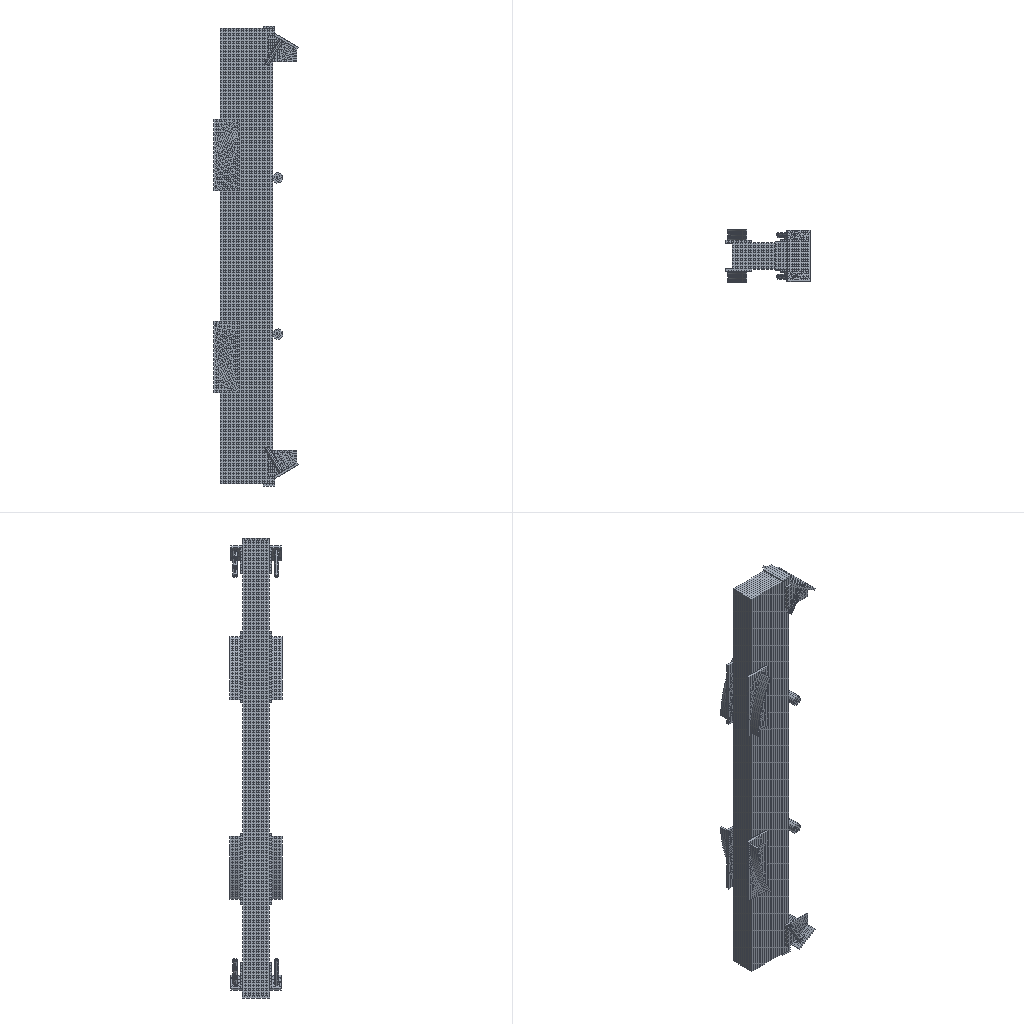Simulation study | abaqus
Set-up summary:
category,name,step,type,value,unit,region
solver,abaqus
solver,version,,,Abaqus/Explicit 2020
units,not stated in the deck,,not stated
analysis,deck,,transient,transient
load_step,Step-1,Step-1,transient
load_step,requested,,,1
mesh,nodes,,,51207
mesh,elements,,,41180
element_type,T3D2,,truss,1847
element_type,C3D8R,,solid,39333
load,load commands in deck,,count,1
bc,support commands in deck,,count,11
material,C40,,in results
material,CFRP,,in results
material,GANGBAN,,in results
material,GANGJIN,,in results
material,GUJIN,,in results
check,setup vs results,,match,"per instance, exact: element labels, types and connectivity; labels of the nodes the elements use; coordinates of those nodes at SINGLE_PRECISION in 10 of 15 instance(s)"
Abaqus input file, long lists of numbers shortened:
*Heading
** Job name: Job-2 Model name: Model-1
** Generated by: Abaqus/CAE 2020
*Preprint, echo=NO, model=NO, history=NO, contact=NO
**
** PARTS
**
*Part, name=ban
*Node
      1,   526.642,  -13.109,         -80.
      2,   526.642,  -23.112,         -80.
** (970 more lines like these left out)
*Element, type=C3D8R
  1, 118, 122, 341, 269,   1,   2,  17,  64
  2, 269, 341, 342, 270,  64,  17,  18,  63
** (441 more lines like these left out)
*Nset, nset=Set-1, generate
   1,  972,    1
*Elset, elset=Set-1, generate
   1,  443,    1
** Section: gangban
*Solid Section, elset=Set-1, material=gangban
,
*End Part
**
*Part, name=ban-Copy
*Node
      1,   507.77,  -151.344,         -80.
      2,   502.692,  -159.959,         -80.
** (960 more lines like these left out)
*Element, type=C3D8R
  1, 118, 122, 341, 269,   1,   2,  17,  64
  2, 269, 341, 342, 270,  64,  17,  18,  63
** (436 more lines like these left out)
*Nset, nset=Set-1, generate
   1,  962,    1
*Elset, elset=Set-1, generate
   1,  438,    1
** Section: gangban
*Solid Section, elset=Set-1, material=gangban
,
*End Part
**
*Part, name=con
*Node
      1,           0.,           0.,           0.
      2,          20.,           0.,           0.
** (40654 more lines like these left out)
*Element, type=C3D8R
    1,   232,   233,   254,   253,     1,     2,    23,    22
    2,   233,   234,   255,   254,     2,     3,    24,    23
** (34998 more lines like these left out)
*Nset, nset=Set-1, generate
     1,  40656,      1
*Elset, elset=Set-1, generate
     1,  35000,      1
** Section: con
*Solid Section, elset=Set-1, material=c40
,
*End Part
**
*Part, name=jin-final
*Node
      1,         365.,        -180.,        3250.
      2,          35.,        -180.,        3250.
** (1401 more lines like these left out)
*Element, type=T3D2
 1,  2, 73
 2, 73, 74
** (1461 more lines like these left out)
*Nset, nset=Set-1
    1,    2,    3,    4,    5,    6,    7,    8,    9,   10,   11,   12,   13,   14,   15,   16
   17,   18,   19,   20,   21,   22,   23,   24,   25,   26,   27,   28,   29,   30,   31,   32
** (54 more lines like these left out)
*Elset, elset=Set-1
   18,   19,   20,   21,   22,   23,   24,   25,   26,   27,   28,   29,   30,   31,   32,   33
   34,   35,   36,   37,   38,   39,   40,   41,   59,   60,   61,   62,   63,   64,   65,   66
** (56 more lines like these left out)
*Nset, nset=Set-2
    1,    2,    3,    5,    7,   10,   11,   12,   13,   14,   15,   16,   17,   18,   19,   20
   21,   22,   23,   24,   25,   26,   27,   28,   29,   30,   31,   32,   33,   34,   35,   36
** (34 more lines like these left out)
*Elset, elset=Set-2
    1,    2,    3,    4,    5,    6,    7,    8,    9,   10,   11,   12,   13,   14,   15,   16
   17,   42,   43,   44,   45,   46,   47,   48,   49,   50,   51,   52,   53,   54,   55,   56
** (32 more lines like these left out)
** Section: gujin
*Solid Section, elset=Set-2, material=gujin
50.5,
** Section: gangjin
*Solid Section, elset=Set-1, material=gangjin
201.,
*End Part
**
*Part, name=mao
*Node
      1,   5.039,   9.778,         220.
      2,   8.131,   15.496,         220.
** (238 more lines like these left out)
*Element, type=C3D8R
  1,  21,  22,  32,  33,   1,   2,  12,  13
  2,  33,  32,  23,  24,  13,  12,   3,   4
** (108 more lines like these left out)
*Nset, nset=Set-1, generate
   1,  240,    1
*Elset, elset=Set-1, generate
   1,  110,    1
** Section: gangban
*Solid Section, elset=Set-1, material=gangban
,
*End Part
**
*Part, name=rig
*Node
      1,   37.278,  -14.504,           0.
      2,   39.879,   3.106,           0.
** (606 more lines like these left out)
*Element, type=C3D8R
  1,  68,  50,  49,  54,  30,  12,  11,  16
  2,  54,  49,  48,  69,  16,  11,  10,  31
** (448 more lines like these left out)
*Nset, nset=Set-1, generate
   1,  608,    1
*Elset, elset=Set-1, generate
   1,  450,    1
** Section: gangban
*Solid Section, elset=Set-1, material=gangban
,
*End Part
**
*Part, name=xian
*Node
      1,  -1897.019,   560.759,           0.
      2,  -1121.676,    103.766,           0.
** (191 more lines like these left out)
*Element, type=T3D2
 1,  2,  7
 2,  7,  8
** (190 more lines like these left out)
*Nset, nset=Set-1, generate
   1,  193,    1
*Elset, elset=Set-1, generate
   1,  192,    1
*Nset, nset=Set-6, generate
   1,  193,    1
*Elset, elset=Set-6, generate
   1,  192,    1
*Orientation, name=Ori-6
          1.,           0.,           0.,           0.,           1.,           0.
1, 0.
** Section: cfrp
*Solid Section, elset=Set-1, material=cfrp
380.,
*End Part
**
*Part, name=zhifan-final
*Node
      1,         416.,           5.,          59.
      2,   424.112,           5.,    45.209
** (2716 more lines like these left out)
*Element, type=C3D8R
  1,  160,  170, 1003,  913,    1,    2,  105,  124
  2,  913, 1003, 1004,  914,  124,  105,  106,  123
** (1229 more lines like these left out)
*Nset, nset=Set-1, generate
    1,  2718,     1
*Elset, elset=Set-1, generate
    1,  1231,     1
** Section: gangban
*Solid Section, elset=Set-1, material=gangban
,
*End Part
**
**
** ASSEMBLY
**
*Assembly, name=Assembly
**
*Instance, name=ban-1, part=ban
        -50.,          20.,         700.
        -50.,          20.,         700., -49.423, 19.423, 700.577,         120.
*End Instance
**
*Instance, name=con-1, part=con
*End Instance
**
*Instance, name=ban-Copy-1, part=ban-Copy
        -50.,          20.,        2250.
        -50.,          20.,        2250., -49.423, 19.423, 2250.577,         120.
*End Instance
**
*Instance, name=ban-2, part=ban
        -50.,        -220.,        2800.
        -50.,        -220.,        2800., -50.577, -219.423, 2800.577,         120.
*End Instance
**
*Instance, name=ban-Copy-2, part=ban-Copy
        -50.,        -220.,        1250.
        -50.,        -220.,        1250., -50.577, -219.423, 1250.577,         120.
*End Instance
**
*Instance, name=rig-1, part=rig
        440.,          50.,        1150.
        440.,          50.,        1150., 441.,          50.,        1150., 90.
*End Instance
**
*Instance, name=rig-1-lin-2-1, part=rig
        440.,          50.,        2350.
        440.,          50.,        2350., 441.,          50.,        2350., 90.
*End Instance
**
*Instance, name=zhifan-final-1, part=zhifan-final
*End Instance
**
*Instance, name=xian-1, part=xian
  -23.419,          60.,  1636.086
  -23.419,          60.,  1636.086, -22.842, 60.577, 1635.508,         120.
*End Instance
**
*Instance, name=xian-1-lin-2-1, part=xian
  -23.419,        -260.,  1636.086
  -23.419,        -260.,  1636.086, -22.842, -259.423, 1635.508,         120.
*End Instance
**
*Instance, name=mao-1, part=mao
354.08, 60., 277.816
354.08, 60., 277.816, 354.08, 61., 277.816, 149.485
*End Instance
**
*Instance, name=mao-1-lin-2-1, part=mao
354.08,        -260., 277.816
354.08,        -260., 277.816, 354.08, -259., 277.816, 149.485
*End Instance
**
*Instance, name=mao-2, part=mao
465.79, 60., 3411.712
465.79, 60., 3411.712, 465.79, 61., 3411.712, 210.515
*End Instance
**
*Instance, name=mao-2-lin-2-1, part=mao
465.79,        -260., 3411.712
465.79,        -260., 3411.712, 465.79, -259., 3411.712, 210.515
*End Instance
**
*Instance, name=jin-final-1, part=jin-final
*End Instance
**
*Node
      1,         400.,        -100.,        1750.
*Nset, nset=Set-3, instance=con-1
     1,    22,    43,    64,    85,   106,   127,   148,   169,   190,   211,   232,   253,   274,   295,   316
   337,   358,   379,   400,   421,   442,   463,   484,   505,   526,   547,   568,   589,   610,   631,   652
** (14 more lines like these left out)
*Elset, elset=Set-3, instance=con-1
     1,    21,    41,    61,    81,   101,   121,   141,   161,   181,   201,   221,   241,   261,   281,   301
   321,   341,   361,   381,   401,   421,   441,   461,   481,   501,   521,   541,   561,   581,   601,   621
** (11 more lines like these left out)
*Nset, nset=Set-4
 1,
*Nset, nset=Set-5, instance=jin-final-1, generate
    1,  1403,     1
*Elset, elset=Set-5, instance=jin-final-1, generate
    1,  1463,     1
*Nset, nset=Set-8, instance=xian-1, generate
   1,  193,    1
*Nset, nset=Set-8, instance=xian-1-lin-2-1, generate
   1,  193,    1
*Elset, elset=Set-8, instance=xian-1, generate
   1,  192,    1
*Elset, elset=Set-8, instance=xian-1-lin-2-1, generate
   1,  192,    1
*Nset, nset=Set-9, instance=xian-1
 1, 6
*Nset, nset=Set-9, instance=xian-1-lin-2-1
 1, 6
*Nset, nset=b_Set-1, instance=rig-1, generate
   1,  608,    1
*Nset, nset=b_Set-1, instance=rig-1-lin-2-1, generate
   1,  608,    1
*Elset, elset=b_Set-1, instance=rig-1, generate
   1,  450,    1
*Elset, elset=b_Set-1, instance=rig-1-lin-2-1, generate
   1,  450,    1
*Nset, nset=m_Set-6, instance=jin-final-1, generate
    1,  1403,     1
*Elset, elset=m_Set-6, instance=jin-final-1, generate
    1,  1463,     1
*Nset, nset=s_Set-6, instance=con-1, generate
     1,  40656,      1
*Elset, elset=s_Set-6, instance=con-1, generate
     1,  35000,      1
*Nset, nset=_PickedSet87, internal
 1,
*Elset, elset=_m_Surf-1_S3, internal, instance=con-1
     1,     2,     3,     4,     5,     6,     7,     8,     9,    10,    11,    12,    13,    14,    15,    16
    17,    18,    19,    20,   201,   202,   203,   204,   205,   206,   207,   208,   209,   210,   211,   212
** (217 more lines like these left out)
*Surface, type=ELEMENT, name=m_Surf-1
_m_Surf-1_S3, S3
*Elset, elset=_m_Surf-4_S5, internal, instance=con-1
   181,   182,   183,   184,   185,   186,   187,   188,   189,   190,   191,   192,   193,   194,   195,   196
   197,   198,   199,   200,   381,   382,   383,   384,   385,   386,   387,   388,   389,   390,   391,   392
** (217 more lines like these left out)
*Surface, type=ELEMENT, name=m_Surf-4
_m_Surf-4_S5, S5
*Elset, elset=_m_Surf-6_S5, internal, instance=con-1
   181,   182,   183,   184,   185,   186,   187,   188,   189,   190,   191,   192,   193,   194,   195,   196
   197,   198,   199,   200,   381,   382,   383,   384,   385,   386,   387,   388,   389,   390,   391,   392
** (217 more lines like these left out)
*Surface, type=ELEMENT, name=m_Surf-6
_m_Surf-6_S5, S5
*Elset, elset=_m_Surf-8_S6, internal, instance=mao-1
   1,   2,   3,   9,  10,  11,  12,  13,  19,  20,  21,  22,  23,  29,  30,  31
  32,  33,  39,  40,  41,  42,  43,  49,  50,  51,  52,  53,  59,  60,  61,  62
** (2 more lines like these left out)
*Elset, elset=_m_Surf-8_S4, internal, instance=mao-1
   4,   5,   6,   7,   8,  14,  15,  16,  17,  18,  24,  25,  26,  27,  28,  34
  35,  36,  37,  38,  44,  45,  46,  47,  48,  54,  55,  56,  57,  58,  64,  65
** (2 more lines like these left out)
*Surface, type=ELEMENT, name=m_Surf-8
_m_Surf-8_S6, S6
_m_Surf-8_S4, S4
*Elset, elset=_m_Surf-10_S6, internal, instance=mao-2
   1,   2,   3,   9,  10,  11,  12,  13,  19,  20,  21,  22,  23,  29,  30,  31
  32,  33,  39,  40,  41,  42,  43,  49,  50,  51,  52,  53,  59,  60,  61,  62
** (2 more lines like these left out)
*Elset, elset=_m_Surf-10_S4, internal, instance=mao-2
   4,   5,   6,   7,   8,  14,  15,  16,  17,  18,  24,  25,  26,  27,  28,  34
  35,  36,  37,  38,  44,  45,  46,  47,  48,  54,  55,  56,  57,  58,  64,  65
** (2 more lines like these left out)
*Surface, type=ELEMENT, name=m_Surf-10
_m_Surf-10_S6, S6
_m_Surf-10_S4, S4
*Elset, elset=_m_Surf-12_S6, internal, instance=mao-2-lin-2-1
   1,   2,   3,   9,  10,  11,  12,  13,  19,  20,  21,  22,  23,  29,  30,  31
  32,  33,  39,  40,  41,  42,  43,  49,  50,  51,  52,  53,  59,  60,  61,  62
** (2 more lines like these left out)
*Elset, elset=_m_Surf-12_S4, internal, instance=mao-2-lin-2-1
   4,   5,   6,   7,   8,  14,  15,  16,  17,  18,  24,  25,  26,  27,  28,  34
  35,  36,  37,  38,  44,  45,  46,  47,  48,  54,  55,  56,  57,  58,  64,  65
** (2 more lines like these left out)
*Surface, type=ELEMENT, name=m_Surf-12
_m_Surf-12_S6, S6
_m_Surf-12_S4, S4
*Elset, elset=_m_Surf-14_S6, internal, instance=mao-1-lin-2-1
   1,   2,   3,   9,  10,  11,  12,  13,  19,  20,  21,  22,  23,  29,  30,  31
  32,  33,  39,  40,  41,  42,  43,  49,  50,  51,  52,  53,  59,  60,  61,  62
** (2 more lines like these left out)
*Elset, elset=_m_Surf-14_S4, internal, instance=mao-1-lin-2-1
   4,   5,   6,   7,   8,  14,  15,  16,  17,  18,  24,  25,  26,  27,  28,  34
  35,  36,  37,  38,  44,  45,  46,  47,  48,  54,  55,  56,  57,  58,  64,  65
** (2 more lines like these left out)
*Surface, type=ELEMENT, name=m_Surf-14
_m_Surf-14_S6, S6
_m_Surf-14_S4, S4
*Elset, elset=_m_Surf-16_S5, internal, instance=zhifan-final-1
 499, 505
*Elset, elset=_m_Surf-16_S4, internal, instance=zhifan-final-1
 503, 520, 556
*Elset, elset=_m_Surf-16_S3, internal, instance=zhifan-final-1
 506, 527
*Elset, elset=_m_Surf-16_S6, internal, instance=zhifan-final-1
 521,
*Surface, type=ELEMENT, name=m_Surf-16
_m_Surf-16_S5, S5
_m_Surf-16_S4, S4
_m_Surf-16_S6, S6
_m_Surf-16_S3, S3
*Elset, elset=_m_Surf-18_S6, internal, instance=zhifan-final-1
 675, 703, 726
*Elset, elset=_m_Surf-18_S5, internal, instance=zhifan-final-1
 678, 683, 689
*Elset, elset=_m_Surf-18_S4, internal, instance=zhifan-final-1
 690, 700
*Surface, type=ELEMENT, name=m_Surf-18
_m_Surf-18_S6, S6
_m_Surf-18_S5, S5
_m_Surf-18_S4, S4
*Elset, elset=_m_Surf-20_S6, internal, instance=mao-2-lin-2-1
   1,   2,   3,   9,  10,  11,  12,  13,  19,  20,  21,  22,  23,  29,  30,  31
  32,  33,  39,  40,  41,  42,  43,  49,  50,  51,  52,  53,  59,  60,  61,  62
** (2 more lines like these left out)
*Elset, elset=_m_Surf-20_S4, internal, instance=mao-2-lin-2-1
   4,   5,   6,   7,   8,  14,  15,  16,  17,  18,  24,  25,  26,  27,  28,  34
  35,  36,  37,  38,  44,  45,  46,  47,  48,  54,  55,  56,  57,  58,  64,  65
** (2 more lines like these left out)
*Surface, type=ELEMENT, name=m_Surf-20
_m_Surf-20_S6, S6
_m_Surf-20_S4, S4
*Elset, elset=_m_Surf-22_S6, internal, instance=mao-2
   1,   2,   3,   9,  10,  11,  12,  13,  19,  20,  21,  22,  23,  29,  30,  31
  32,  33,  39,  40,  41,  42,  43,  49,  50,  51,  52,  53,  59,  60,  61,  62
** (2 more lines like these left out)
*Elset, elset=_m_Surf-22_S4, internal, instance=mao-2
   4,   5,   6,   7,   8,  14,  15,  16,  17,  18,  24,  25,  26,  27,  28,  34
  35,  36,  37,  38,  44,  45,  46,  47,  48,  54,  55,  56,  57,  58,  64,  65
** (2 more lines like these left out)
*Surface, type=ELEMENT, name=m_Surf-22
_m_Surf-22_S6, S6
_m_Surf-22_S4, S4
*Elset, elset=_m_Surf-24_S6, internal, instance=zhifan-final-1
 1157, 1158, 1160, 1164, 1165, 1167, 1171, 1172, 1174, 1178, 1179, 1181, 1185, 1186, 1188, 1192
 1193, 1195, 1199, 1200, 1202, 1206, 1207, 1209, 1213, 1214, 1216, 1220, 1221, 1223, 1227, 1228
** (1 more lines like these left out)
*Elset, elset=_m_Surf-24_S1, internal, instance=zhifan-final-1
  309,  310,  311,  312,  313,  314,  315,  316,  317,  318,  319,  320,  321,  322,  323,  324
  325,  326,  327,  328,  329,  330,  331,  332,  333,  334,  335,  336,  337,  338,  339,  340
** (6 more lines like these left out)
*Elset, elset=_m_Surf-24_S5, internal, instance=zhifan-final-1
 1155, 1156, 1161, 1162, 1163, 1168, 1169, 1170, 1175, 1176, 1177, 1182, 1183, 1184, 1189, 1190
 1191, 1196, 1197, 1198, 1203, 1204, 1205, 1210, 1211, 1212, 1217, 1218, 1219, 1224, 1225, 1226
** (1 more lines like these left out)
*Surface, type=ELEMENT, name=m_Surf-24
_m_Surf-24_S6, S6
_m_Surf-24_S1, S1
_m_Surf-24_S5, S5
*Elset, elset=_m_Surf-26_S1, internal, instance=zhifan-final-1
 111, 112, 113, 114, 115, 116, 117, 118, 119, 120, 121, 122, 123, 124, 125, 126
 127, 128, 129, 130, 131, 132, 133, 134, 135, 136, 137, 138, 139, 140, 141, 142
** (6 more lines like these left out)
*Elset, elset=_m_Surf-26_S5, internal, instance=zhifan-final-1
 739, 740, 745, 746, 747, 752, 753, 754, 759, 760, 761, 766, 767, 768, 773, 774
 775, 780, 781, 782, 787, 788, 789, 794, 795, 796, 801, 802, 803, 808, 809, 810
** (1 more lines like these left out)
*Elset, elset=_m_Surf-26_S6, internal, instance=zhifan-final-1
 741, 742, 744, 748, 749, 751, 755, 756, 758, 762, 763, 765, 769, 770, 772, 776
 777, 779, 783, 784, 786, 790, 791, 793, 797, 798, 800, 804, 805, 807, 811, 812
** (1 more lines like these left out)
*Surface, type=ELEMENT, name=m_Surf-26
_m_Surf-26_S1, S1
_m_Surf-26_S5, S5
_m_Surf-26_S6, S6
*Elset, elset=_m_Surf-27_S4, internal, instance=rig-1
   1,   2,  15,  26,  31,  32,  45,  56,  61,  62,  75,  86,  91,  92, 105, 116
 121, 122, 135, 146, 151, 152, 165, 176, 181, 182, 195, 206, 211, 212, 225, 236
** (2 more lines like these left out)
*Elset, elset=_m_Surf-27_S6, internal, instance=rig-1
   9,  11,  14,  17,  39,  41,  44,  47,  69,  71,  74,  77,  99, 101, 104, 107
 129, 131, 134, 137, 159, 161, 164, 167, 189, 191, 194, 197, 219, 221, 224, 227
** (2 more lines like these left out)
*Elset, elset=_m_Surf-27_S3, internal, instance=rig-1
  10,  19,  20,  25,  40,  49,  50,  55,  70,  79,  80,  85, 100, 109, 110, 115
 130, 139, 140, 145, 160, 169, 170, 175, 190, 199, 200, 205, 220, 229, 230, 235
** (2 more lines like these left out)
*Elset, elset=_m_Surf-27_S5, internal, instance=rig-1
  13,  18,  43,  48,  73,  78, 103, 108, 133, 138, 163, 168, 193, 198, 223, 228
 253, 258, 283, 288, 313, 318, 343, 348, 373, 378, 403, 408, 433, 438
*Surface, type=ELEMENT, name=m_Surf-27
_m_Surf-27_S4, S4
_m_Surf-27_S6, S6
_m_Surf-27_S3, S3
_m_Surf-27_S5, S5
*Elset, elset=_m_Surf-29_S4, internal, instance=rig-1-lin-2-1
   1,   2,  15,  26,  31,  32,  45,  56,  61,  62,  75,  86,  91,  92, 105, 116
 121, 122, 135, 146, 151, 152, 165, 176, 181, 182, 195, 206, 211, 212, 225, 236
** (2 more lines like these left out)
*Elset, elset=_m_Surf-29_S6, internal, instance=rig-1-lin-2-1
   9,  11,  14,  17,  39,  41,  44,  47,  69,  71,  74,  77,  99, 101, 104, 107
 129, 131, 134, 137, 159, 161, 164, 167, 189, 191, 194, 197, 219, 221, 224, 227
** (2 more lines like these left out)
*Elset, elset=_m_Surf-29_S3, internal, instance=rig-1-lin-2-1
  10,  19,  20,  25,  40,  49,  50,  55,  70,  79,  80,  85, 100, 109, 110, 115
 130, 139, 140, 145, 160, 169, 170, 175, 190, 199, 200, 205, 220, 229, 230, 235
** (2 more lines like these left out)
*Elset, elset=_m_Surf-29_S5, internal, instance=rig-1-lin-2-1
  13,  18,  43,  48,  73,  78, 103, 108, 133, 138, 163, 168, 193, 198, 223, 228
 253, 258, 283, 288, 313, 318, 343, 348, 373, 378, 403, 408, 433, 438
*Surface, type=ELEMENT, name=m_Surf-29
_m_Surf-29_S4, S4
_m_Surf-29_S6, S6
_m_Surf-29_S3, S3
_m_Surf-29_S5, S5
*Elset, elset=_m_Surf-30_S6, internal, instance=ban-1, generate
   1,  100,    1
*Surface, type=ELEMENT, name=m_Surf-30
_m_Surf-30_S6, S6
*Elset, elset=_m_Surf-32_S6, internal, instance=ban-Copy-1, generate
   1,  100,    1
*Surface, type=ELEMENT, name=m_Surf-32
_m_Surf-32_S6, S6
*Elset, elset=_m_Surf-34_S6, internal, instance=ban-Copy-2, generate
   1,  100,    1
*Surface, type=ELEMENT, name=m_Surf-34
_m_Surf-34_S6, S6
*Elset, elset=_m_Surf-36_S6, internal, instance=ban-2, generate
   1,  100,    1
*Surface, type=ELEMENT, name=m_Surf-36
_m_Surf-36_S6, S6
*Elset, elset=_s_Surf-1_S2, internal, instance=ban-1, generate
 101,  443,    1
*Surface, type=ELEMENT, name=s_Surf-1
_s_Surf-1_S2, S2
*Elset, elset=_s_Surf-3_S2, internal, instance=ban-Copy-1, generate
 101,  438,    1
*Surface, type=ELEMENT, name=s_Surf-3
_s_Surf-3_S2, S2
*Elset, elset=_s_Surf-4_S2, internal, instance=ban-Copy-2, generate
 101,  438,    1
*Surface, type=ELEMENT, name=s_Surf-4
_s_Surf-4_S2, S2
*Elset, elset=_s_Surf-6_S2, internal, instance=ban-2, generate
 101,  443,    1
*Surface, type=ELEMENT, name=s_Surf-6
_s_Surf-6_S2, S2
*Elset, elset=_s_Surf-8_, internal, instance=xian-1, generate
 148,  192,    1
*Surface, type=ELEMENT, name=s_Surf-8
_s_Surf-8_,
*Elset, elset=_s_Surf-10_, internal, instance=xian-1, generate
  1,  45,   1
*Surface, type=ELEMENT, name=s_Surf-10
_s_Surf-10_,
*Elset, elset=_s_Surf-12_, internal, instance=xian-1-lin-2-1, generate
  1,  45,   1
*Surface, type=ELEMENT, name=s_Surf-12
_s_Surf-12_,
*Elset, elset=_s_Surf-14_, internal, instance=xian-1-lin-2-1, generate
 148,  192,    1
*Surface, type=ELEMENT, name=s_Surf-14
_s_Surf-14_,
*Elset, elset=_s_Surf-16_, internal, instance=xian-1-lin-2-1, generate
 148,  192,    1
*Surface, type=ELEMENT, name=s_Surf-16
_s_Surf-16_,
*Elset, elset=_s_Surf-18_, internal, instance=xian-1, generate
 148,  192,    1
*Surface, type=ELEMENT, name=s_Surf-18
_s_Surf-18_,
*Elset, elset=_s_Surf-20_, internal, instance=xian-1-lin-2-1, generate
  1,  45,   1
*Surface, type=ELEMENT, name=s_Surf-20
_s_Surf-20_,
*Elset, elset=_s_Surf-22_, internal, instance=xian-1, generate
  1,  45,   1
*Surface, type=ELEMENT, name=s_Surf-22
_s_Surf-22_,
*Elset, elset=_s_Surf-24_S4, internal, instance=con-1, generate
    20,  35000,     20
*Elset, elset=_s_Surf-24_S5, internal, instance=con-1
   181,   182,   183,   184,   185,   186,   187,   188,   189,   190,   191,   192,   193,   194,   195,   196
   197,   198,   199,   200,   381,   382,   383,   384,   385,   386,   387,   388,   389,   390,   391,   392
** (217 more lines like these left out)
*Elset, elset=_s_Surf-24_S3, internal, instance=con-1
     1,     2,     3,     4,     5,     6,     7,     8,     9,    10,    11,    12,    13,    14,    15,    16
    17,    18,    19,    20,   201,   202,   203,   204,   205,   206,   207,   208,   209,   210,   211,   212
** (217 more lines like these left out)
*Elset, elset=_s_Surf-24_S1, internal, instance=con-1, generate
 34801,  35000,      1
*Surface, type=ELEMENT, name=s_Surf-24
_s_Surf-24_S4, S4
_s_Surf-24_S5, S5
_s_Surf-24_S3, S3
_s_Surf-24_S1, S1
*Elset, elset=_s_Surf-27_S4, internal, instance=con-1, generate
    20,  35000,     20
*Surface, type=ELEMENT, name=s_Surf-27
_s_Surf-27_S4, S4
*Elset, elset=_s_Surf-30_, internal, instance=xian-1, generate
 123,  147,    1
*Surface, type=ELEMENT, name=s_Surf-30
_s_Surf-30_,
*Elset, elset=_s_Surf-32_, internal, instance=xian-1, generate
 46,  70,   1
*Surface, type=ELEMENT, name=s_Surf-32
_s_Surf-32_,
*Elset, elset=_s_Surf-34_, internal, instance=xian-1-lin-2-1, generate
 123,  147,    1
*Surface, type=ELEMENT, name=s_Surf-34
_s_Surf-34_,
*Elset, elset=_s_Surf-36_, internal, instance=xian-1-lin-2-1, generate
 46,  70,   1
*Surface, type=ELEMENT, name=s_Surf-36
_s_Surf-36_,
** Constraint: Constraint-1
*Tie, name=Constraint-1, adjust=yes
s_Surf-1, m_Surf-1
** Constraint: Constraint-2
*Tie, name=Constraint-2, adjust=yes
s_Surf-3, m_Surf-1
** Constraint: Constraint-3
*Tie, name=Constraint-3, adjust=yes
s_Surf-4, m_Surf-4
** Constraint: Constraint-4
*Tie, name=Constraint-4, adjust=yes
s_Surf-6, m_Surf-6
** Constraint: Constraint-5
*Tie, name=Constraint-5, adjust=yes
s_Surf-8, m_Surf-8
** Constraint: Constraint-6
*Tie, name=Constraint-6, adjust=yes
s_Surf-10, m_Surf-10
** Constraint: Constraint-7
*Tie, name=Constraint-7, adjust=yes
s_Surf-12, m_Surf-12
** Constraint: Constraint-8
*Tie, name=Constraint-8, adjust=yes
s_Surf-14, m_Surf-14
** Constraint: Constraint-10
*Tie, name=Constraint-10, adjust=yes
s_Surf-16, m_Surf-16
** Constraint: Constraint-11
*Tie, name=Constraint-11, adjust=yes
s_Surf-18, m_Surf-18
** Constraint: Constraint-12
*Tie, name=Constraint-12, adjust=yes
s_Surf-20, m_Surf-20
** Constraint: Constraint-13
*Tie, name=Constraint-13, adjust=yes
s_Surf-22, m_Surf-22
** Constraint: Constraint-14
*Tie, name=Constraint-14, adjust=yes
s_Surf-24, m_Surf-24
** Constraint: Constraint-15
*Tie, name=Constraint-15, adjust=yes
s_Surf-24, m_Surf-26
** Constraint: Constraint-neizhi
*Embedded Element, host elset=s_Set-6
m_Set-6
** Constraint: Constraint-rig
*Rigid Body, ref node=_PickedSet87, elset=b_Set-1
*End Assembly
*Amplitude, name=Amp-1
             0.,              0.,             0.1,              1.
**
** MATERIALS
**
*Material, name=c40
*Density
 2.5e-09,
*Elastic
32500., 0.2
*Concrete Damaged Plasticity
30.,   0.1,  1.16, 0.667,  0.01
*Concrete Compression Hardening
 31.839,          0.
  35.238, 0.0001688
  37.656, 0.0002734
 39.058, 0.0004092
    39.5, 0.0005746
 38.815, 0.0007747
 37.101,  0.001006
  34.823,  0.001256
 32.332,  0.001511
 29.849,  0.001767
 27.497,  0.002018
 25.334,   0.002263
 23.376,  0.002503
 21.619,  0.002736
 20.051,  0.002963
 18.651,  0.003185
 17.402,  0.003403
 16.285,  0.003616
 15.284,  0.003826
 14.385,   0.004032
 13.573,  0.004236
 12.839,  0.004438
 12.173,  0.004637
 11.567,   0.004835
  11.013,  0.005031
*Concrete Tension Stiffening
  2.09,       0.
   2.4, 8.74e-06
  2.67, 1.23e-05
  2.86, 1.81e-05
  2.94, 2.75e-05
   2.8, 4.37e-05
  2.55, 6.31e-05
   2.3, 8.27e-05
  2.07, 0.000102
  1.86,  0.00012
  1.69, 0.000137
  1.55, 0.000153
  1.42, 0.000169
  1.31, 0.000184
  1.22, 0.000198
  1.14, 0.000213
  1.07, 0.000227
  1.01,  0.00024
 0.956, 0.000254
 0.908, 0.000267
 0.864,  0.00028
 0.825, 0.000293
 0.789, 0.000306
 0.757, 0.000319
 0.727, 0.000332
*Concrete Compression Damage
        0.,          0.
 0.06977, 0.0001688
  0.1005, 0.0002734
  0.1363, 0.0004092
  0.176, 0.0005746
  0.2212, 0.0007747
  0.271,  0.001006
  0.3214,  0.001256
  0.3699,  0.001511
  0.4151,  0.001767
  0.4565,  0.002018
  0.4939,   0.002263
  0.5275,  0.002503
   0.5577,  0.002736
  0.5849,  0.002963
   0.6093,  0.003185
  0.6313,  0.003403
  0.6511,  0.003616
  0.6691,  0.003826
  0.6855,   0.004032
  0.7004,  0.004236
  0.7141,  0.004438
  0.7266,  0.004637
  0.7382,   0.004835
  0.7488,  0.005031
  0.7586,  0.005226
  0.7678,  0.005419
  0.7763,  0.005611
  0.7842,  0.005802
  0.7915,  0.005993
  0.7984,  0.006182
  0.8049,  0.006371
  0.811,  0.006559
  0.8167,  0.006747
  0.8221,  0.006933
  0.8627,  0.008781
  0.8884,   0.01061
  0.906,   0.01242
  0.9188,   0.01423
  0.9286,   0.01603
** (21 more lines like these left out)
*Concrete Tension Damage, compression recovery=0.45
     0.,       0.
 0.0544, 8.74e-06
 0.0674, 1.23e-05
 0.0893, 1.81e-05
  0.124, 2.75e-05
  0.186, 4.37e-05
  0.255, 6.31e-05
  0.321, 8.27e-05
   0.38, 0.000102
  0.431,  0.00012
  0.475, 0.000137
  0.513, 0.000153
  0.546, 0.000169
  0.575, 0.000184
  0.601, 0.000198
  0.623, 0.000213
  0.643, 0.000227
  0.661,  0.00024
  0.678, 0.000254
  0.692, 0.000267
  0.706,  0.00028
  0.718, 0.000293
  0.729, 0.000306
  0.739, 0.000319
  0.749, 0.000332
  0.757, 0.000344
  0.765, 0.000357
  0.773, 0.000369
   0.78, 0.000382
  0.787, 0.000394
  0.793, 0.000407
  0.799, 0.000419
  0.804, 0.000431
  0.809, 0.000443
  0.814, 0.000456
  0.851, 0.000577
  0.875, 0.000697
  0.892, 0.000816
  0.905, 0.000935
  0.915,  0.00105
** (31 more lines like these left out)
*Material, name=cfrp
*Density
 1.8e-09,
*Elastic
160000., 0.25
*Material, name=gangban
*Density
 7.8e-09,
*Elastic
210000., 0.3
*Plastic
235.,0.
*Material, name=gangjin
*Density
 7.8e-09,
*Elastic
196700., 0.2
*Plastic
 451.1,      0.
 604.5, 0.00878
*Material, name=gujin
*Density
 7.8e-09,
*Elastic
201300., 0.2
*Plastic
 447.8,  0.
 619.7, 0.1
**
** INTERACTION PROPERTIES
**
*Surface Interaction, name=IntProp-1
*Friction
 0.2,
*Surface Behavior, pressure-overclosure=HARD
*Surface Interaction, name=IntProp-2
*Friction
 0.1,
*Surface Behavior, pressure-overclosure=HARD
**
** PREDEFINED FIELDS
**
** Name: Predefined Field-1   Type: Stress
*Initial Conditions, type=STRESS
Set-5, -5., -5., -5.,
** Name: Predefined Field-2   Type: Stress
*Initial Conditions, type=STRESS
Set-8, -50., -50., -50.,
** ----------------------------------------------------------------
**
** STEP: Step-1
**
*Step, name=Step-1, nlgeom=YES
*Dynamic, Explicit
, 0.1
*Bulk Viscosity
0.06, 1.2
**
** BOUNDARY CONDITIONS
**
** Name: BC-1 Type: 位移/转角
*Boundary
Set-3, 1, 1
Set-3, 2, 2
Set-3, 4, 4
Set-3, 6, 6
** Name: BC-3 Type: 对称/反对称/完全固定
*Boundary
Set-9, ENCASTRE
** Name: [REDACTED] : Displacement/rotation angle
*Boundary, amplitude=Amp-1
Set-4, 1, 1, -30.
Set-4, 2, 2
Set-4, 3, 3
Set-4, 4, 4
Set-4, 5, 5
Set-4, 6, 6
**
** INTERACTIONS
**
** Interaction: Int-1
*Contact Pair, interaction=IntProp-1, mechanical constraint=KINEMATIC, cpset=Int-1
m_Surf-27, s_Surf-27
** Interaction: Int-1-Copy
*Contact Pair, interaction=IntProp-1, mechanical constraint=KINEMATIC, cpset=Int-1-Copy
m_Surf-29, s_Surf-27
** Interaction: Int-3
*Contact, op=NEW
*Contact Inclusions, ALL EXTERIOR
*Contact Property Assignment
 ,  , IntProp-2
**
** OUTPUT REQUESTS
**
*Restart, write, number interval=1, time marks=NO
**
** FIELD OUTPUT: F-Output-1
**
*Output, field, number interval=50
*Node Output
A, CF, RF, RM, RT, U, V
*Element Output, directions=YES
DAMAGEC, DAMAGET, E, EVF, LE, MISES, MISESMAX, MISESONLY, PE, PEEQ, PEEQMAX, PEEQT, PEEQVAVG, PEMAG, PEVAVG, S
SDEG, SEQUT, SF, SSAVG, SVAVG, VEEQ, YIELDPOT
*Contact Output
CDISP, CFORCE, CSTRESS
**
** HISTORY OUTPUT: H-Output-1
**
*Output, history, time interval=2e-06
*Node Output, nset=Set-4
RF1, U1
*End Step
Results summary:
result,step,Step-1,completed,increments=110148 time=0.1/0.1
result,analysis,,,transient
result,last_loadstep,,,1
result,primary field,,,U
result,reaction total,,FX,-3319.21,model units
result,reaction total,,FY,9541.873,model units
result,reaction total,,FZ,1451.145,model units